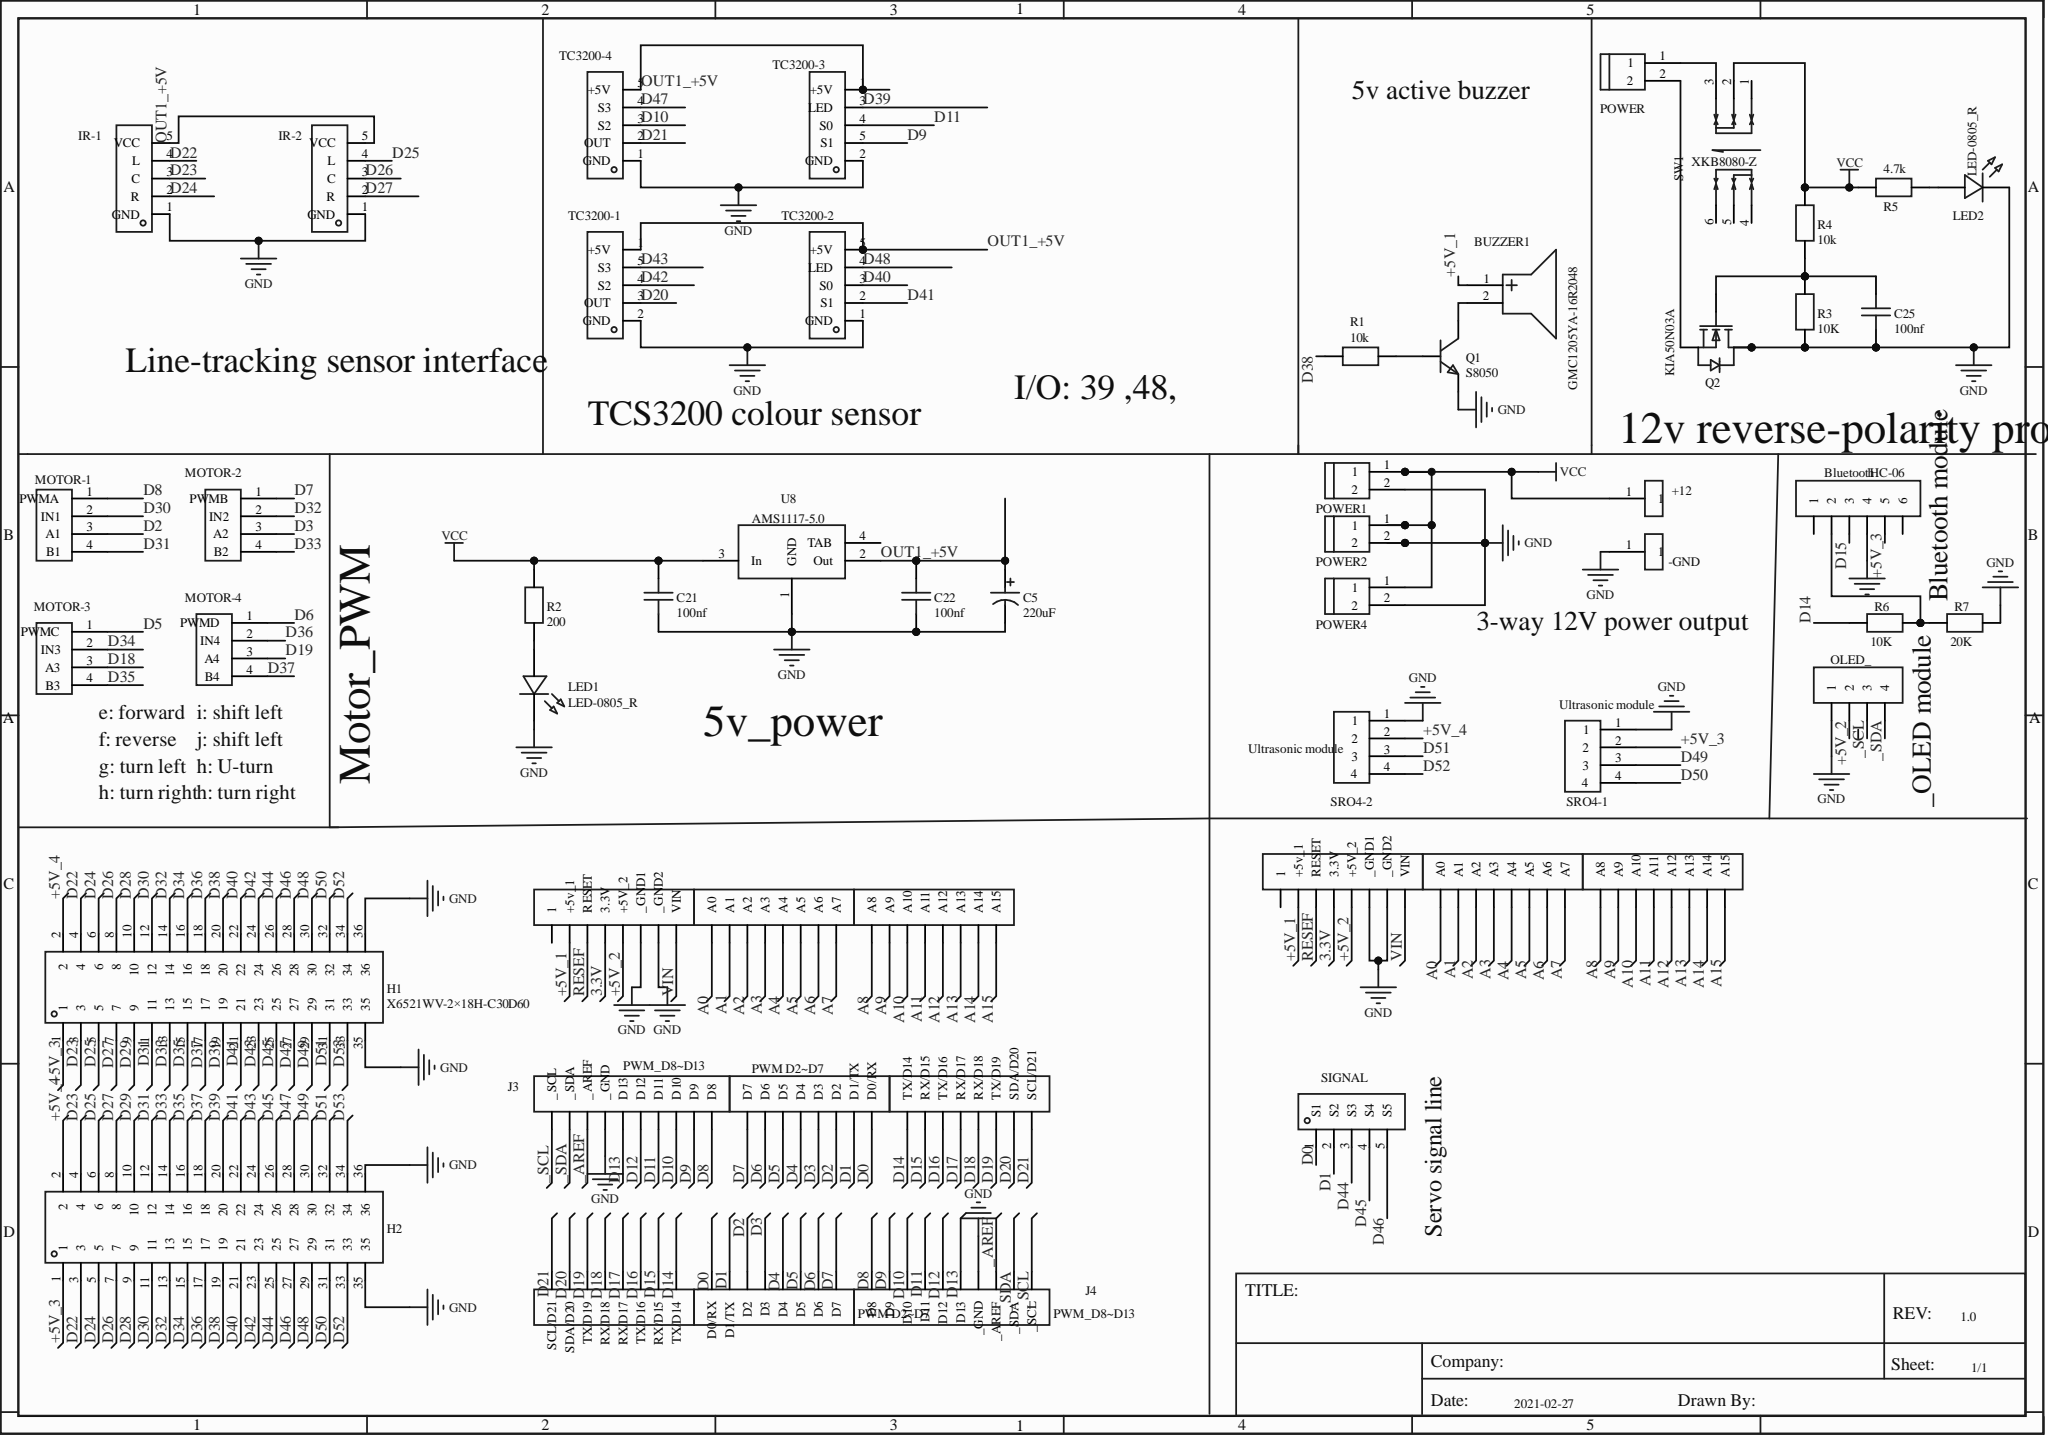Circuit board | Altium Designer | 53 parts | 91 nets
Bill of materials:
Comment,Description,Designator,Footprint,LibRef,Quantity
"Pad","","+12, -GND","焊盘","焊盘","2"
"GMC1205YA-16R2048","","BUZZER1","BUZ-TH_BD12.0-P6.50-D0.6-FD","GMC1205YA-16R2048","1"
"220uF","","C5","","CK1A221M-CRE54","1"
"100nf","","C21, C22, C25","C0603","100nf","3"
"X6521WV-2×18H-C30D60","","H1, H2","HDR-TH_36P-2.54-V-M-R2-C18-S2.54","X6521WV-2×18H-C30D60","2"
"Bluetooth","","HC-06","HDR-F-2.54_1X6","蓝牙","1"
"XH-5A_C722874","","IR-1, IR-2, SIGNAL, TC3200-1, TC3200-2, TC3200-3, TC3200-4","CONN-TH_XH-5A","XH-5A","7"
"3-way TX/RX","","J1, J6","HDR-M-2.54_1X8","3路TX/RX","2"
"PWM D2~D7","","J2, J5","HDR-M-2.54_1X8","PWM D2~D7","2"
"PWM_D8~D13","","J3, J4","HDR-M-2.54_1X10","PWM_D8~D13","2"
"HDR-M-2.54_1x8","","J7, J8, J9, J12, J13, J14","HDR-M-2.54_1X8","HDR-M-2.54_1x8","6"
"LED-0805_R","","LED1, LED2","LED0805_RED","17-21SURC/S530-A3/TR8","2"
"MOTOR-1","","MOTOR-1","CONN-TH_4P-P2.50_XH-4A","XH-4A","1"
"MOTOR-2","","MOTOR-2","CONN-TH_4P-P2.50_XH-4A","XH-4A","1"
"MOTOR-3","","MOTOR-3","CONN-TH_4P-P2.50_XH-4A","XH-4A","1"
"MOTOR-4","","MOTOR-4","CONN-TH_4P-P2.50_XH-4A","XH-4A","1"
"OLED_","","OLED-","HDR-F-2.54_1X4","OLED_","1"
"XH-2AW","","POWER, POWER1, POWER2, POWER4","CONN-TH_2P-P2.50_XH-2AW","XH-2AW","4"
"S8050","","Q1","SOT-23-3_L2.9-W1.3-P1.90-LS2.4-BR","S8050","1"
"KIA50N03A","","Q2","TO-252-2_L6.6-W6.1-P4.57-LS9.9-TL-CW","KIA50N03A","1"
"10k","","R1, R3, R4, R6","R0603","10k","4"
"200","","R2","R0603","200","1"
"4.7k","","R5","R0603","4.7k","1"
"20K","","R7","R0603","20K","1"
"Ultrasonic module","","SRO4-1, SRO4-2","CONN-TH_4P-P2.50_XH-4A","XH-4A","2"
"XKB8080-Z","","SW1","SW-TH_6P-L8.0-W8.0-P2.50","XKB8080-Z","1"
"AMS1117-5.0","","U8","SOT-223_L6.5-W3.5-P2.30-LS7.0-BR","AMS1117-5.0","1"
Netlist (Protel format):
[
+12
焊盘
Pad



]
[
-GND
焊盘
Pad



]
[
BUZZER1
BUZ-TH_BD12.0-P6.50-D0.6-FD
GMC1205YA-16R2048



]
[
C5

220uF



]
[
C21
C0603
100nf



]
[
C22
C0603
100nf



]
[
C25
C0603
100nf



]
[
H1
HDR-TH_36P-2.54-V-M-R2-C18-S2.54
X6521WV-2×18H-C30D60



]
[
H2
HDR-TH_36P-2.54-V-M-R2-C18-S2.54
X6521WV-2×18H-C30D60



]
[
HC-06
HDR-F-2.54_1X6
Bluetooth



]
[
IR-1
CONN-TH_XH-5A
XH-5A_C722874



]
[
IR-2
CONN-TH_XH-5A
XH-5A_C722874



]
[
J1
HDR-M-2.54_1X8
3-way TX/RX



]
[
J2
HDR-M-2.54_1X8
PWM D2~D7



]
[
J3
HDR-M-2.54_1X10
PWM_D8~D13



]
[
J4
HDR-M-2.54_1X10
PWM_D8~D13



]
[
J5
HDR-M-2.54_1X8
PWM D2~D7



]
[
J6
HDR-M-2.54_1X8
3-way TX/RX



]
[
J7
HDR-M-2.54_1X8
HDR-M-2.54_1x8



]
[
J8
HDR-M-2.54_1X8
HDR-M-2.54_1x8



]
[
J9
HDR-M-2.54_1X8
HDR-M-2.54_1x8



]
[
J12
HDR-M-2.54_1X8
HDR-M-2.54_1x8



]
[
J13
HDR-M-2.54_1X8
HDR-M-2.54_1x8



]
[
J14
HDR-M-2.54_1X8
HDR-M-2.54_1x8



]
[
LED1
LED0805_RED
LED-0805_R



]
[
LED2
LED0805_RED
LED-0805_R



]
[
MOTOR-1
CONN-TH_4P-P2.50_XH-4A
MOTOR-1



]
[
MOTOR-2
CONN-TH_4P-P2.50_XH-4A
MOTOR-2



]
[
MOTOR-3
CONN-TH_4P-P2.50_XH-4A
MOTOR-3



]
[
MOTOR-4
CONN-TH_4P-P2.50_XH-4A
MOTOR-4



]
[
OLED-
HDR-F-2.54_1X4
OLED_



]
[
POWER
CONN-TH_2P-P2.50_XH-2AW
XH-2AW



]
[
POWER1
CONN-TH_2P-P2.50_XH-2AW
XH-2AW



]
[
POWER2
CONN-TH_2P-P2.50_XH-2AW
XH-2AW



]
[
POWER4
CONN-TH_2P-P2.50_XH-2AW
XH-2AW



]
[
Q1
SOT-23-3_L2.9-W1.3-P1.90-LS2.4-BR
S8050



]
[
Q2
TO-252-2_L6.6-W6.1-P4.57-LS9.9-TL-CW
KIA50N03A



]
[
R1
R0603
10k



]
[
R2
R0603
200



]
[
R3
R0603
10K



]
[
R4
R0603
10k



]
[
R5
R0603
4.7k



]
[
R6
R0603
10K



]
[
R7
R0603
20K



]
[
SIGNAL
CONN-TH_XH-5A
XH-5A_C722874



]
[
SRO4-1
CONN-TH_4P-P2.50_XH-4A
Ultrasonic module



]
[
SRO4-2
CONN-TH_4P-P2.50_XH-4A
Ultrasonic module



]
[
SW1
SW-TH_6P-L8.0-W8.0-P2.50
XKB8080-Z



]
[
TC3200-1
CONN-TH_XH-5A
XH-5A_C722874



]
[
TC3200-2
CONN-TH_XH-5A
XH-5A_C722874



]
[
TC3200-3
CONN-TH_XH-5A
XH-5A_C722874



]
[
TC3200-4
CONN-TH_XH-5A
XH-5A_C722874



]
[
U8
SOT-223_L6.5-W3.5-P2.30-LS7.0-BR
AMS1117-5.0



]
(
VIN
J9-8
J12-8
)
(
VCC
+12-1
C21-2
POWER1-1
POWER2-1
POWER4-1
R2-2
R4-1
R5-1
SW1-2
U8-3
)
(
RESEF
J9-3
J12-3
)
(
OUT1_+5V
C5-1
C22-2
IR-1-5
IR-2-5
TC3200-1-1
TC3200-2-5
TC3200-3-1
TC3200-4-5
U8-2
)
(
NetQ1_1
Q1-1
R1-2
)
(
NetPOWER_2
POWER-2
Q2-3
)
(
NetPOWER_1
POWER-1
SW1-3
)
(
NetLED2_1
LED2-1
R5-2
)
(
NetLED1_1
LED1-1
R2-1
)
(
NetHC-06_2
HC-06-2
R6-1
R7-2
)
(
NetC25_2
C25-2
Q2-1
R3-2
R4-2
)
(
NetBUZZER1_2
BUZZER1-2
Q1-3
)
(
GND
-GND-1
C5-2
C21-1
C22-1
C25-1
H1-35
H1-36
H2-35
H2-36
HC-06-4
IR-1-1
IR-2-1
J3-4
J4-4
J9-6
J9-7
J12-6
J12-7
LED1-2
LED2-2
OLED--1
POWER1-2
POWER2-2
POWER4-2
Q1-2
Q2-2
R3-1
R7-1
SRO4-1-1
SRO4-2-1
TC3200-1-2
TC3200-2-1
TC3200-3-2
TC3200-4-1
U8-1
)
(
D53
H1-33
H2-34
)
(
D52
H1-34
H2-33
SRO4-2-4
)
(
D51
H1-31
H2-32
SRO4-2-3
)
(
D50
H1-32
H2-31
SRO4-1-4
)
(
D49
H1-29
H2-30
SRO4-1-3
)
(
D48
H1-30
H2-29
TC3200-2-4
)
(
D47
H1-27
H2-28
TC3200-4-4
)
(
D46
H1-28
H2-27
SIGNAL-5
)
(
D45
H1-25
H2-26
SIGNAL-4
)
(
D44
H1-26
H2-25
SIGNAL-3
)
(
D43
H1-23
H2-24
TC3200-1-5
)
(
D42
H1-24
H2-23
TC3200-1-4
)
(
D41
H1-21
H2-22
TC3200-2-2
)
(
D40
H1-22
H2-21
TC3200-2-3
)
(
D39
H1-19
H2-20
TC3200-3-3
)
(
D38
H1-20
H2-19
R1-1
)
(
D37
H1-17
H2-18
MOTOR-4-4
)
(
D36
H1-18
H2-17
MOTOR-4-2
)
(
D35
H1-15
H2-16
MOTOR-3-4
)
(
D34
H1-16
H2-15
MOTOR-3-2
)
(
D33
H1-13
H2-14
MOTOR-2-4
)
(
D32
H1-14
H2-13
MOTOR-2-2
)
(
D31
H1-11
H2-12
MOTOR-1-4
)
(
D30
H1-12
H2-11
MOTOR-1-2
)
(
D29
H1-9
H2-10
)
(
D28
H1-10
H2-9
)
(
D27
H1-7
H2-8
IR-2-2
)
(
D26
H1-8
H2-7
IR-2-3
)
(
D25
H1-5
H2-6
IR-2-4
)
(
D24
H1-6
H2-5
IR-1-2
)
(
D23
H1-3
H2-4
IR-1-3
)
(
D22
H1-4
H2-3
IR-1-4
)
(
D21
J1-8
J6-8
TC3200-4-2
)
(
D20
J1-7
J6-7
TC3200-1-3
)
(
D19
J1-6
J6-6
MOTOR-4-3
)
(
D18
J1-5
J6-5
MOTOR-3-3
)
(
D17
J1-4
J6-4
)
(
D16
J1-3
J6-3
)
(
D15
HC-06-3
J1-2
J6-2
)
(
D14
J1-1
J6-1
R6-2
)
(
D13
J3-5
J4-5
)
(
D12
J3-6
J4-6
)
(
D11
J3-7
J4-7
TC3200-3-4
)
(
D10
J3-8
J4-8
TC3200-4-3
)
(
D9
J3-9
J4-9
TC3200-3-5
)
(
D8
J3-10
J4-10
MOTOR-1-1
)
(
D7
J2-1
J5-1
MOTOR-2-1
)
(
D6
J2-2
J5-2
MOTOR-4-1
)
(
D5
J2-3
J5-3
MOTOR-3-1
)
(
D4
J2-4
J5-4
)
(
D3
J2-5
J5-5
MOTOR-2-3
)
(
D2
J2-6
J5-6
MOTOR-1-3
)
(
D1
J2-7
J5-7
SIGNAL-2
)
(
D0
J2-8
J5-8
SIGNAL-1
)
(
A15
J7-8
J14-8
)
(
A14
J7-7
J14-7
)
(
A13
J7-6
J14-6
)
(
A12
J7-5
J14-5
)
(
A11
J7-4
J14-4
)
(
A10
J7-3
J14-3
)
(
A9
J7-2
J14-2
)
(
A8
J7-1
J14-1
)
(
A7
J8-8
J13-8
)
(
A6
J8-7
J13-7
)
(
A5
J8-6
J13-6
)
(
A4
J8-5
J13-5
)
(
A3
J8-4
J13-4
)
(
A2
J8-3
J13-3
)
(
A1
J8-2
J13-2
)
(
A0
J8-1
J13-1
)
(
_SDA
J3-2
J4-2
OLED--4
)
(
_SCL
J3-1
J4-1
OLED--3
)
(
_AREF
J3-3
J4-3
)
(
+5V_4
H1-2
H2-2
SRO4-2-2
)
(
+5V_3
H1-1
H2-1
HC-06-5
SRO4-1-2
)
(
+5V_2
J9-5
J12-5
OLED--2
)
(
+5V_1
BUZZER1-1
J9-2
J12-2
)
(
3.3V
J9-4
J12-4
)